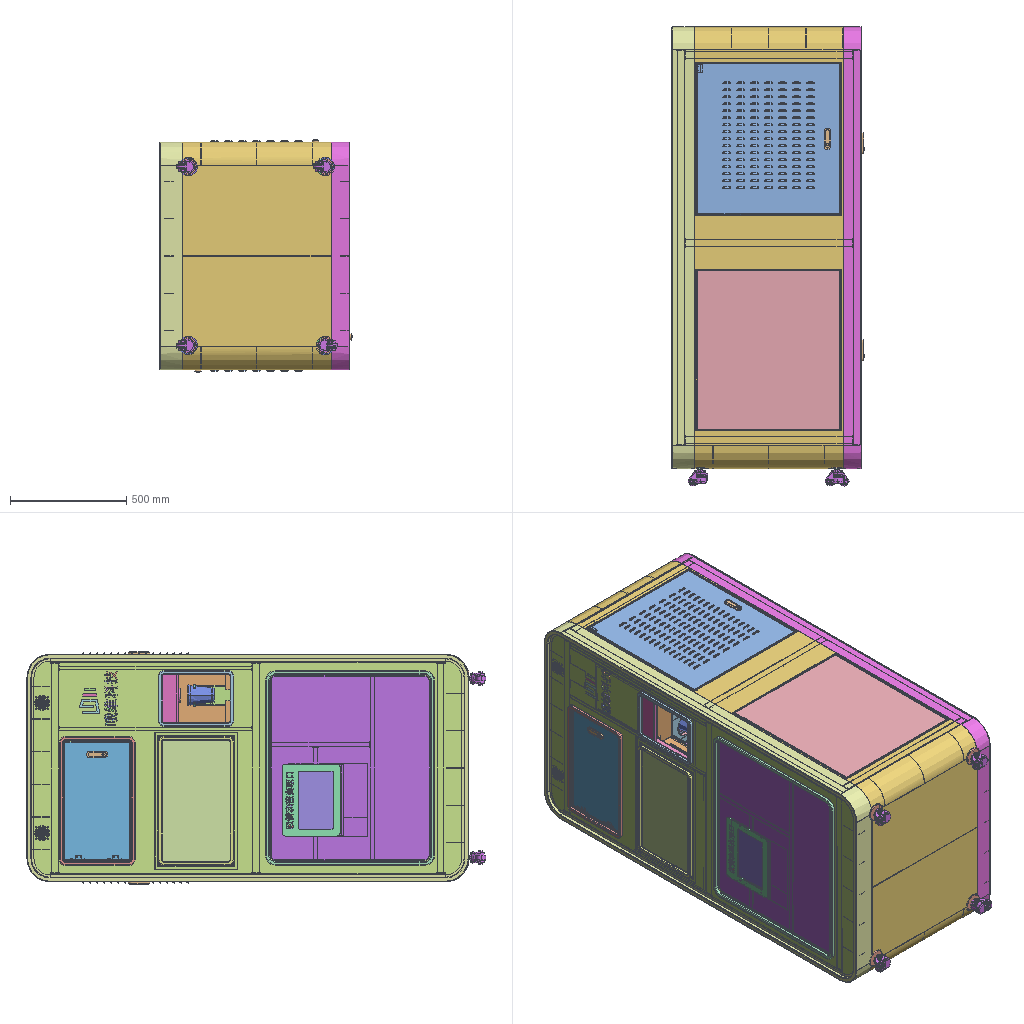Assembly | STEP file | 137 different items | 347 placed | box 826 x 1977 x 1000 mm
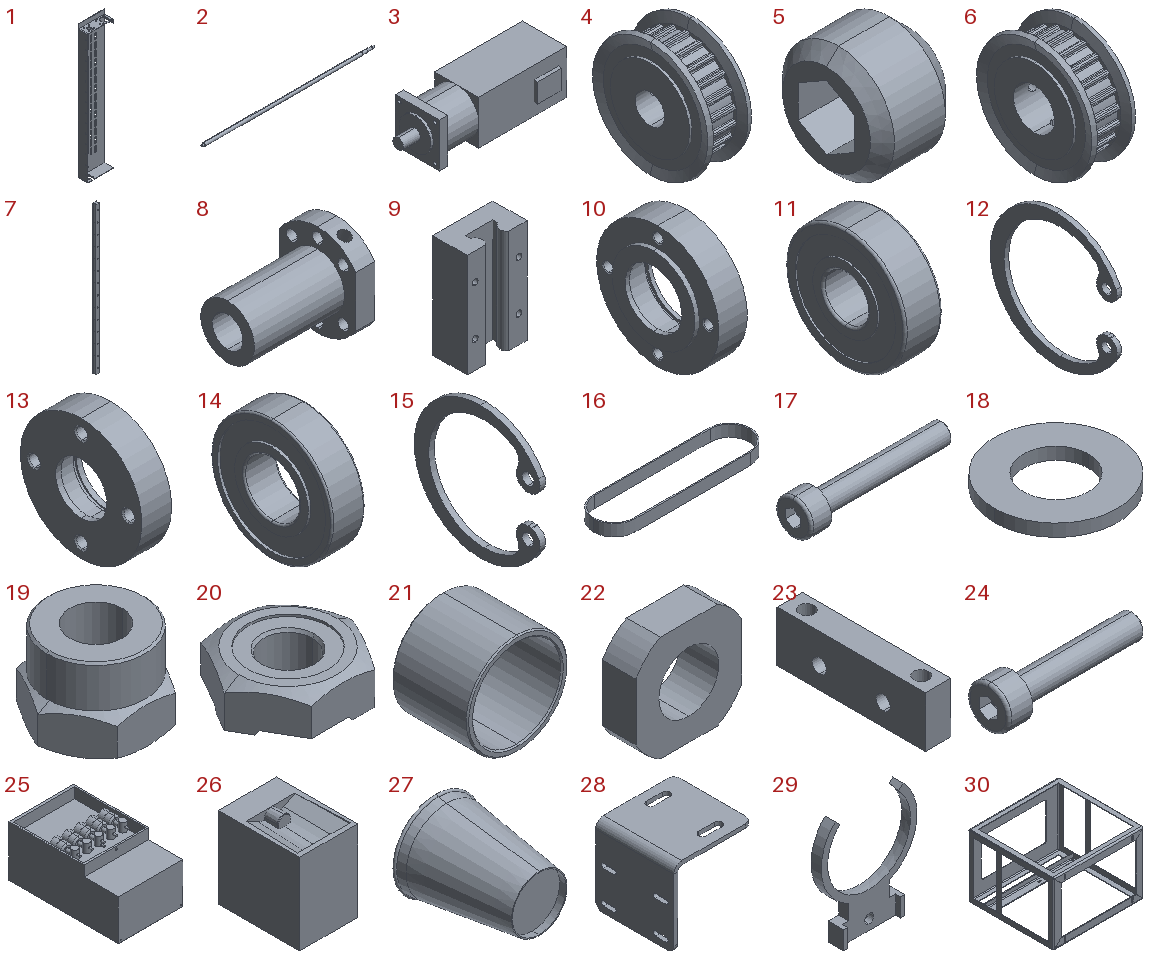Parts list (item | name | quantity | parent item | size | volume):
1 | Lead screw mechanism sheet metal V1.201001 | x1 | in Translation drive module V1.201001 | 175 x 65 x 885 mm | 405761 mm3
2 | Lead screw 16V1.201001 | x1 | in Translation drive module V1.201001 | 882 x 16 x 16 mm | 170889 mm3
3 | PX57N005S0 planetary reducer+motor V1.201001 | x1 | in Translation drive module V1.201001 | 193 x 63 x 58 mm | 546492 mm3
4 | Synchronous wheel TTPA22-AT5100-A-P10_b V1.201001 | x1 | in Synchronous wheel TTPA22-AT5100-A-P10 V1.201001 | 15 x 40 x 40 mm | 11899 mm3
5 | Synchronous wheel SET-SCREW4-3V1.201001 | x2 | in Synchronous wheel TTPA22-AT5100-A-P10 V1.201001 | 3 x 4 x 4 mm | 27.73 mm3
6 | Synchronous wheel shaft 14V1.201001 | x1 | in Translation drive module V1.201001 | 15 x 40 x 40 mm | 10801 mm3
7 | Linear guide rail HG20 V1.201001 | x1 | in Translation drive module V1.201001 | 20 x 18 x 840 mm | 247602 mm3
8 | Lead screw nut SFU01610-3V1.201001 | x1 | in Translation drive module V1.201001 | 57 x 40 x 48 mm | 32254 mm3
9 | Linear slider HGH20CA V1.201001 | x1 | in Translation drive module V1.201001 | 44 x 25 x 76 mm | 66387 mm3
10 | Bearing seat BARR6201DD_b V1.201001 | x1 | in Round flange bearing seat BARR6201 V1.201001 | 15 x 56 x 56 mm | 21210 mm3
11 | Bearing seat bearing_6201 V1.201001 | x1 | in Round flange bearing seat BARR6201 V1.201001 | 10 x 32 x 32 mm | 6608 mm3
12 | Bearing seat RRING-C-INT-32V1.201001 | x1 | in Round flange bearing seat BARR6201 V1.201001 | 1.2 x 32.2 x 33.7 mm | 309.422 mm3
13 | Bearing seat BGRAB6900DD_h V1.201001 | x1 | in Round flange bearing seat BGRAB6900 V1.201001 | 11 x 45 x 45 mm | 12216 mm3
14 | Bearing seat bearing_6900 V1.201001 | x1 | in Round flange bearing seat BGRAB6900 V1.201001 | 6 x 22 x 22 mm | 1661 mm3
15 | Bearing seat RRING-C-INT-22V1.201001 | x1 | in Round flange bearing seat BGRAB6900 V1.201001 | 1 x 21.856 x 23 mm | 128.626 mm3
16 | Belt V1.201001 | x1 | in Translation drive module V1.201001 | 136 x 36 x 10 mm | 3100 mm3
17 | hexagon socket head cap screws gbV1.201001_GB_FASTENER_SCREWS_HSHCS M4X25-N | x3 | in Translation drive module V1.201001 | 29 x 7 x 7 mm | 449.083 mm3
18 | plain washers-n series-grade a gbV1.201001_GB_FASTENER_WASHER_PWNA 5 | x4 | in Translation drive module V1.201001, Coffee machine | 10 x 10 x 1 mm | 56.478 mm3
19 | prevailing torque type style 1 gbV1.201001_GB_HEXAGON_TYPE9 M5-N | x4 | in Translation drive module V1.201001, Coffee machine | 9.238 x 8 x 6.8 mm | 245.877 mm3
20 | hexagon weld nuts gb01001_GB_FASTENER_NUT_JSCN M5-N | x2 | in Translation drive module V1.201001 | 11.547 x 10 x 4 mm | 240.353 mm3
21 | Lead screw shaft end spacer V1.201001 | x1 | in Translation drive module V1.201001 | 16 x 12 x 16 mm | 561.717 mm3
22 | - | x1 | in Translation drive module V1.201001 | 22 x 8 x 22 mm | 2378 mm3
23 | Belt tensioner seat 1001 | x1 | in Translation drive module V1.201001 | 6 x 35 x 12 mm | 2186 mm3
24 | Hex socket cap screw M4 X 20_GB_FASTENER_SCREWS_HSHCS M4X20-N | x1 | in Translation drive module V1.201001 | 24 x 7 x 7 mm | 386.251 mm3
25 | Beverage coffee machine V1.201001 | x1 | in Coffee machine | 430 x 730 x 364 mm | 89425555 mm3
26 | Ice maker V1.201001 | x2 | in Coffee machine | 250 x 350 x 351.956 mm | 29308107 mm3
27 | Paper cup V1.201001 | x2 | in Coffee machine | 92.598 x 112 x 92.598 mm | 30103 mm3
28 | Drive module fixing part V1.201001 | x2 | in Coffee machine | 60 x 60 x 59 mm | 23708 mm3
29 | Cup gripper V1.201001 | x1 | in Coffee machine | 94 x 15 x 108.734 mm | 27097 mm3
30 | Ice maker bracket V1.201001 | x1 | in Coffee machine | 360 x 340 x 250 mm | 395832 mm3
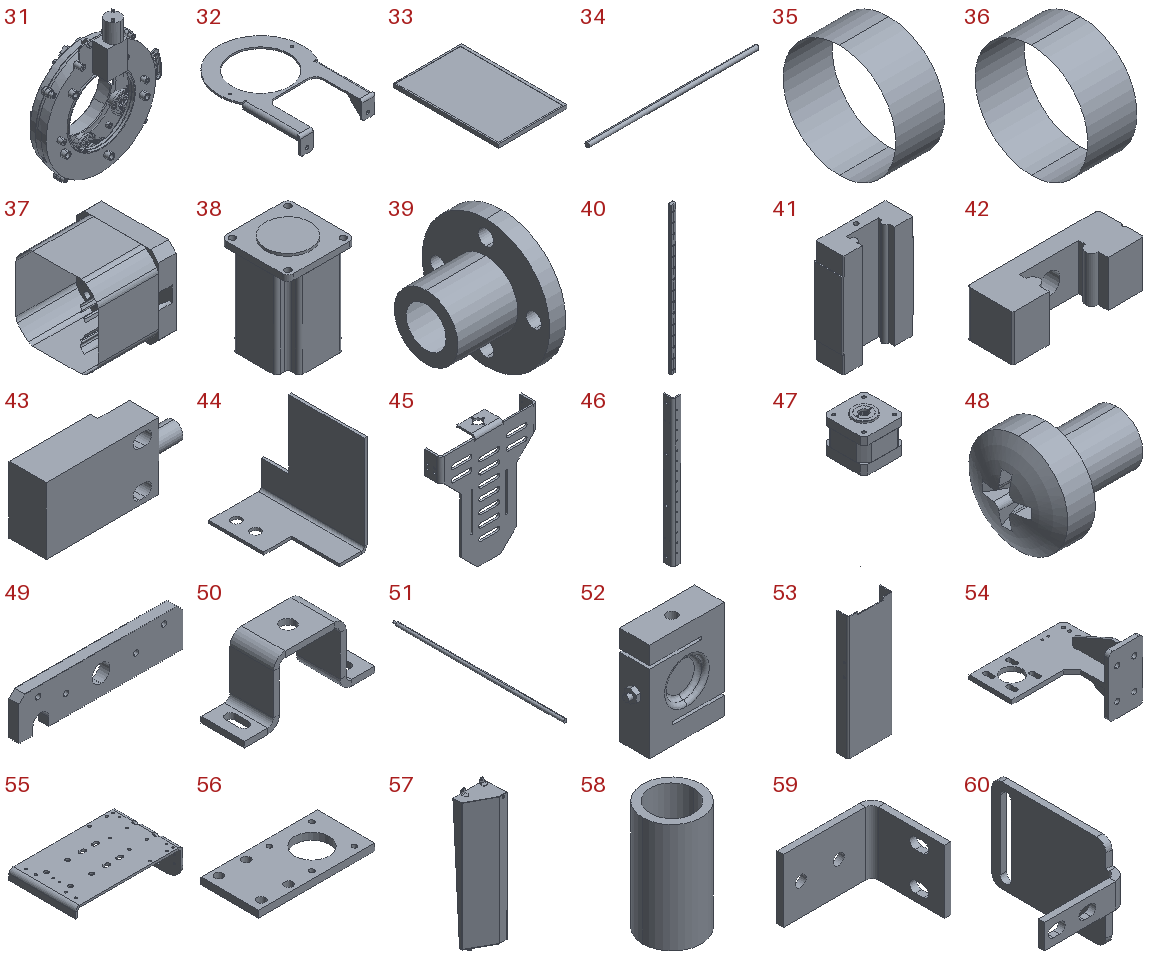31 | 90-bore adjustable cup dropper with cup bucket assembly V1.201001 | x1 | in Coffee machine | - | 341072 mm3
32 | Cup dropper fixing bracket V1.201001 | x1 | in Coffee machine | 160 x 225.6 x 35 mm | 51040 mm3
33 | Operation moving screen V1.201001 | x1 | in Coffee machine | 232 x 356 x 12.5 mm | 957215 mm3
34 | Lift screen drive 42-48-T8-100L_1 V1.201001 | x1 | in Lift screen drive 42-48-T8-100L V1.201001 | - | -
35 | Lift screen drive 42-48-T8-100L_3 V1.201001 | x1 | in Lift screen drive 42-48-T8-100L V1.201001 | - | -
36 | Lift screen drive 42-48-T8-100L_4 V1.201001 | x1 | in Lift screen drive 42-48-T8-100L V1.201001 | - | -
37 | Lift screen drive 42-48-T8-100L_6 V1.201001 | x1 | in Lift screen drive 42-48-T8-100L V1.201001 | - | -
38 | 57 stepper motor 001 | x1 | in Lift screen drive 42-48-T8-100L V1.201001 | 57 x 57 x 80 mm | 221641 mm3
39 | Lead screw nut T10001 | x1 | in Lift screen drive 42-48-T8-100L V1.201001 | - | -
40 | MANIFOLD_SOLID_BREP_106V1.201001 | x2 | in MGN9CV1.201001 | 9 x 6.5 x 300 mm | 14670 mm3
41 | MGN9C slider V1.201001 | x4 | in MGN9CV1.201001, MGN9C for cup gripper 1001, Coffee machine | 20 x 8 x 28.9 mm | 3300 mm3
42 | MGN9 limit block 1001 | x4 | in MGN9CV1.201001 | 20 x 7 x 7 mm | 695.088 mm3
43 | Photoelectric proximity switch V1.201001 | x4 | in Coffee machine | 38.5 x 10.5 x 18.5 mm | 5130 mm3
44 | Proximity switch bracket 3V1.201001 | x1 | in Coffee machine | 20 x 37.5 x 36 mm | 1594 mm3
45 | Lift screen fixing plate V1.201001 | x1 | in Coffee machine | 211 x 40 x 250 mm | 134618 mm3
46 | Guide rail bracket V1.201001 | x2 | in Coffee machine | 18 x 22 x 330 mm | 34095 mm3
47 | 42HSC1409-250NE2V1.201001 | x1 | in Through-type lead screw motor 42HSC1409-250NE2 V1.201001 | 42.3 x 47.3 x 139 mm | 58209 mm3
48 | cross recessed pan head screws gb_GB_CROSS_SCREWS_TYPE1 M3X4-4  H type-NV1.201001 | x4 | in Through-type lead screw motor 42HSC1409-250NE2 V1.201001 | 6.37 x 5.6 x 5.6 mm | 73.791 mm3
49 | Load cell connecting block V1.201001 | x1 | in Coffee lift drive module V1.201001 | 82 x 5 x 20 mm | 7453 mm3
50 | Lead screw connecting block V1.201001 | x1 | in Coffee lift drive module V1.201001 | 45 x 15 x 22 mm | 2255 mm3
51 | Tr8 lead screw V1.201001 | x1 | in Coffee lift drive module V1.201001 | 8 x 388 x 8 mm | 19201 mm3
52 | Load cell JLBS-1V1.201001 | x1 | in Coffee machine | 56 x 20 x 66 mm | 60086 mm3
53 | Upper stop plate V1.201001 | x1 | in Coffee machine | 86 x 23 x 240 mm | 45312 mm3
54 | Lead screw guide rail connecting plate split 1V1.201001 | x1 | in Coffee machine | 110 x 92.5 x 70 mm | 52117 mm3
55 | Lead screw guide rail connecting plate split 2V1.201001 | x1 | in Coffee machine | 161 x 100 x 44.931 mm | 60540 mm3
56 | Lead screw motor drive mounting plate split V1.201001 | x1 | in Coffee machine | 85 x 42 x 5 mm | 14638 mm3
57 | Sink bevel V1.201001 | x1 | in Coffee machine sink bevel V1.201001 | 200 x 147.478 x 872.907 mm | 358159 mm3
58 | Drain pipe weld joint V1.201001 | x1 | in Coffee machine sink bevel V1.201001 | 16 x 16 x 30 mm | 2639 mm3
59 | Cup gripper lift proximity switch bracket 01V1.201001 | x1 | in Coffee machine | 30 x 25 x 20 mm | 1957 mm3
60 | Cup gripper lift proximity switch bracket 02V1.201001 | x1 | in Coffee machine | 27 x 42 x 30 mm | 2421 mm3
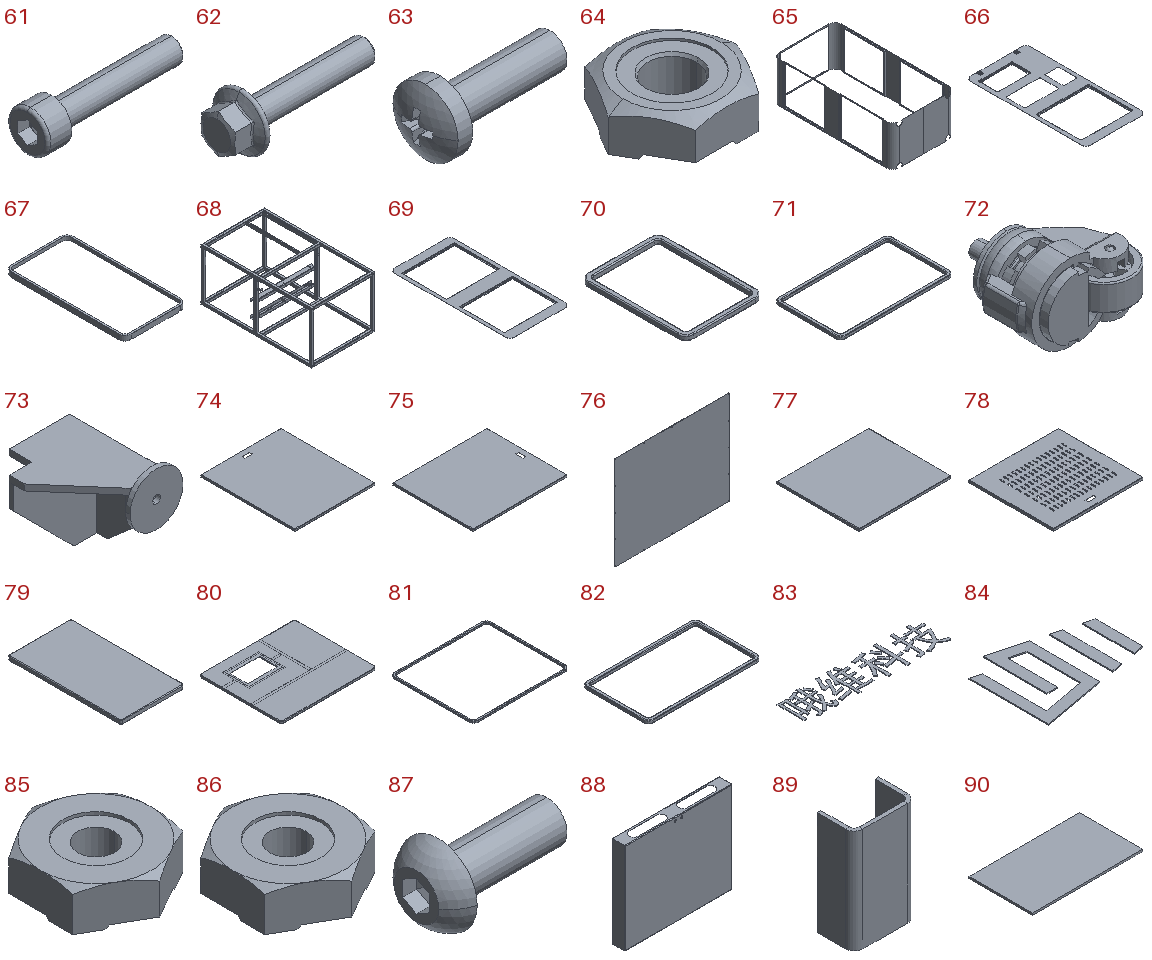61 | hexagon socket head cap screws gbV1.201001_GB_FASTENER_SCREWS_HSHCS M5X25-N | x1 | in Coffee machine | 30 x 8.5 x 8.5 mm | 732.65 mm3
62 | hexagon flange bolts--small series gbV1.201001_GB_FASTENER_BOLT_HFBSS M5X25-N | x1 | in Coffee machine | 30.6 x 11.4 x 11.4 mm | 799.257 mm3
63 | cross recessed pan head screws gbV1.201001_GB_CROSS_SCREWS_TYPE1 M5X16-16  H type-N | x4 | in Coffee machine | 19.658 x 9.5 x 9.5 mm | 509.153 mm3
64 | hexagon weld nuts gbV1.201001_GB_FASTENER_NUT_JSCN M5-N | x2 | in Coffee machine | 11.547 x 10 x 4 mm | 240.353 mm3
65 | Split housing part 0101001 | x1 | in Split arc housing 01001 | 980 x 1900 x 640 mm | 2630768 mm3
66 | Split housing part 0201001 | x1 | in Split arc housing 01001 | 920 x 1840 x 21.5 mm | 1371751 mm3
67 | Split housing part 0301001 | x1 | in Split arc housing 01001 | 980 x 1900 x 80 mm | 894741 mm3
68 | Coffee machine structure frame 01001_default<by machining> | x1 | in Split arc housing 01001 | 977 x 1697 x 797 mm | 7192337 mm3
69 | Split housing part 0401001 | x1 | in Split arc housing 01001 | 920 x 1840 x 21.5 mm | 1137707 mm3
70 | Lift screen decorative outer frame 001001 | x1 | in Split arc housing 01001 | 240 x 325 x 16 mm | 57771 mm3
71 | 23.6 inch transparent screen outer fixing frame 001001 | x1 | in Split arc housing 01001 | 554 x 325 x 16 mm | 92756 mm3
72 | Fuma wheel 60S01001 | x4 | in Split arc housing 01001 | 82.6 x 87.32 x 58 mm | 125258 mm3
73 | Foot support 01001 | x4 | in Split arc housing 01001 | 129 x 131 x 129 mm | 250060 mm3
74 | Rear door panel V1.201001 | x1 | in Split arc housing 01001 | 686 x 805 x 19 mm | 939207 mm3
75 | Rear door panel lower V1.201001 | x1 | in Split arc housing 01001 | 805 x 686 x 19 mm | 939207 mm3
76 | Top cover plate V1.201001 | x1 | in Split arc housing 01001 | 780 x 1.5 x 640 mm | 748466 mm3
77 | Side door panel lower V1.201001 | x2 | in Split arc housing 01001 | 686 x 615 x 19 mm | 731060 mm3
78 | Side door panel upper V1.201001 | x2 | in Split arc housing 01001 | 651 x 615 x 25 mm | 711845 mm3
79 | Front small door panel V1.201001 | x1 | in Split arc housing 01001 | 285 x 511 x 19 mm | 277788 mm3
80 | Front door panel lower V1.201001_default<by machining> | x1 | in Split arc housing 01001 | 796 x 686 x 21.5 mm | 1058682 mm3
81 | Front door outer fixing frame lower 01001 | x1 | in Split arc housing 01001 | 836 x 726 x 16 mm | 745654 mm3
82 | Front small door fixing frame 01001 | x1 | in Split arc housing 01001 | 554 x 325 x 16 mm | 92756 mm3
83 | COMPANY_A 01001 | x1 | in Split arc housing 01001 | 232.982 x 55.205 x 1 mm | 4335 mm3
84 | COMPANY_A LOGO01001 | x1 | in Split arc housing 01001 | 110 x 87.475 x 1 mm | 3655 mm3
85 | Hex weld nut M3_DIN 929-M3-N | x16 | in Split arc housing 01001 | 7.5 x 8.66 x 3 mm | 111.431 mm3
86 | Hex weld nut M3_DIN 929-M3-N | x48 | in Split arc housing 01001 | 7.5 x 8.66 x 3 mm | 111.431 mm3
87 | Hex socket flat round head screw M3 X 8_GB_SOCKET_TYPE7 M3X8-N | x16 | in Split arc housing 01001 | 9.65 x 5.7 x 5.7 mm | 82.74 mm3
88 | Electrical cabinet V1.201001 | x1 | in Split arc housing 01001 | 813 x 100 x 693 mm | 1252271 mm3
89 | Reinforcing rib 1001 | x6 | in Split arc housing 01001 | 25 x 15 x 42 mm | 3127 mm3
90 | 23.6 inch glass 001 | x1 | in Split arc housing 01001 | 550 x 315 x 10 mm | 1732500 mm3
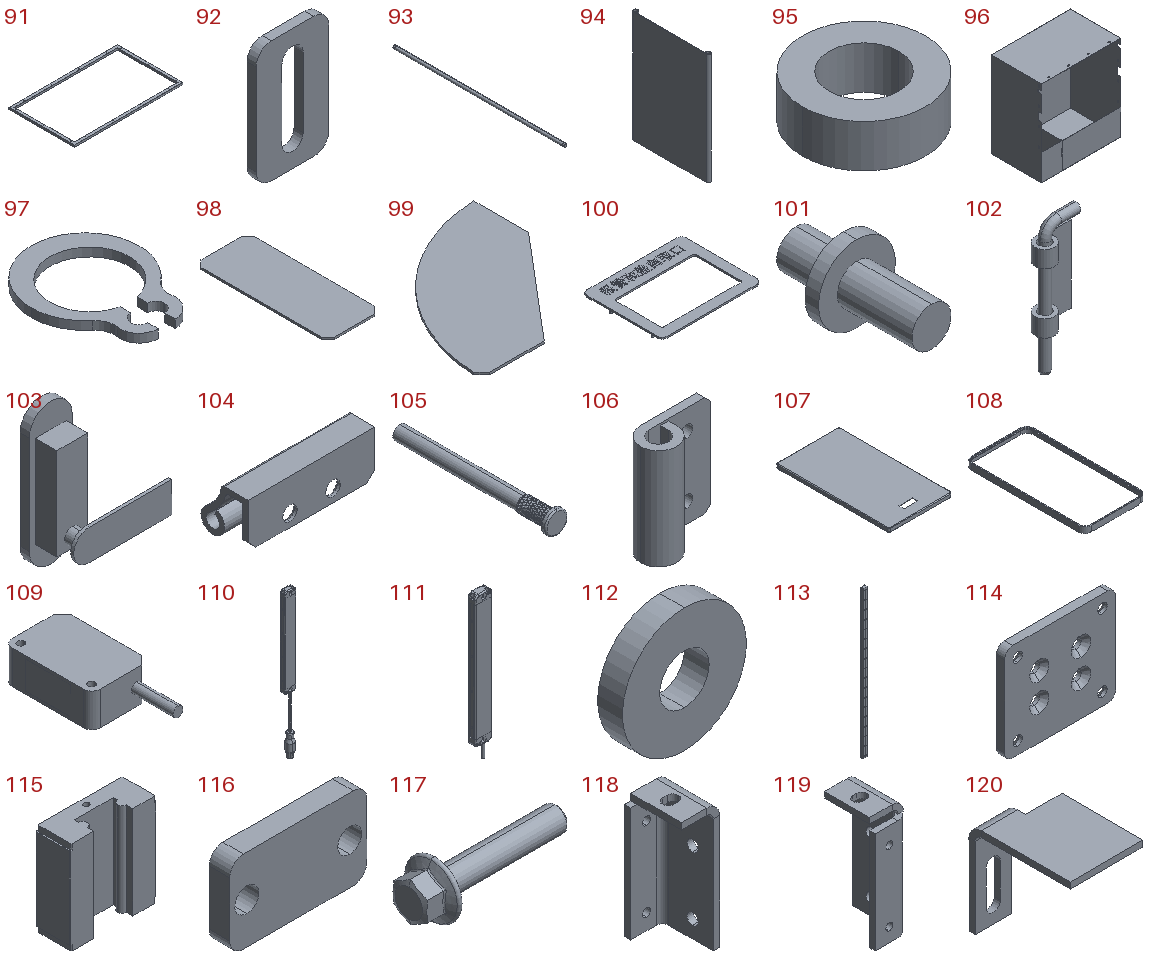91 | Glass mouth reinforcing frame 001 | x1 | in Split arc housing 01001 | 590 x 355 x 11 mm | 93227 mm3
92 | Glass fixing block 001 | x14 | in Split arc housing 01001 | 12 x 1.5 x 20 mm | 277.146 mm3
93 | 6mm pin shaft 001 | x1 | in Split arc housing 01001 | 6 x 320 x 6 mm | 9038 mm3
94 | Coffee machine cover door panel 001 | x1 | in Split arc housing 01001 | 10 x 180 x 260 mm | 84055 mm3
95 | Flip door spacer 001 | x2 | in Split arc housing 01001 | 11.5 x 11.5 x 4 mm | 282.743 mm3
96 | Lid storage box 001 | x1 | in Split arc housing 01001 | 315 x 200 x 340 mm | 428432 mm3
97 | circlips for shaft--type a small gb001_GB_CONNECTING_PIECE_RING_RRA 6 | x2 | in Split arc housing 01001 | 7.6 x 9.565 x 0.6 mm | 14.427 mm3
98 | Box reinforcing rib plate 001 | x22 | in Split arc housing 01001 | 40 x 100 x 1.5 mm | 5925 mm3
99 | Box reinforcing rib plate 2001 | x16 | in Split arc housing 01001 | 94.931 x 99.938 x 1.5 mm | 8426 mm3
100 | Straw and lid self-pickup opening 001 | x1 | in Split arc housing 01001 | 310 x 250 x 20.1 mm | 200534 mm3
101 | Hinge lower door shaft 001 | x4 | in Split arc housing 01001 | 7.8 x 13.8 x 7.8 mm | 219.742 mm3
102 | Latch hinge 001 | x4 | in Split arc housing 01001 | 17.5 x 10 x 55 mm | 2208 mm3
103 | Door lock KL-MS77-1001 | x5 | in Split arc housing 01001 | 68 x 35 x 92 mm | 37880 mm3
104 | - | x2 | in Hinge CL237001 | 48.5 x 18 x 18 mm | 3837 mm3
105 | - | x2 | in Hinge CL237001 | 8 x 57 x 8 mm | 1212 mm3
106 | - | x2 | in Hinge CL237001 | 20 x 9 x 25 mm | 1667 mm3
107 | Front small door panel mating hinge leaf 001 | x1 | in Split arc housing 01001 | 285 x 511 x 19 mm | 270507 mm3
108 | Housing front face solid 001 | x1 | in Split arc housing 01001 | 980 x 1900 x 96 mm | 1146713 mm3
109 | BGS photoelectric switch PG6 V1.201001 | x2 | in Coffee machine | 21 x 46.5 x 12 mm | 7794 mm3
110 | Safety light curtain 4PLN-0440-P V1.201001 | x1 | in Coffee machine | 22.25 x 14.5 x 284 mm | 22094 mm3
111 | Safety light curtain 4PLN-0440V1.201001 | x1 | in Coffee machine | 22 x 10 x 192 mm | 17011 mm3
112 | Guide rail bracket shim 1001 | x7 | in Coffee machine | 10 x 2 x 10 mm | 131.947 mm3
113 | MGN9 guide rail 1001 | x2 | in MGN9C for cup gripper 1001, Coffee machine | 9 x 6.5 x 350 mm | 17052 mm3
114 | MGN9C slider mounting base plate 1001 | x2 | in Coffee machine | 40 x 3 x 35 mm | 3776 mm3
115 | MGN9S slider 1001 | x2 | in Coffee machine | 20 x 8 x 21.5 mm | 2522 mm3
116 | MGN9C short slider pad plate 1001 | x2 | in Coffee machine | 20 x 3 x 12 mm | 651.972 mm3
117 | Hex flange bolt small series M5 X 25_GB_FASTENER_BOLT_HFBSS M5X25-N | x2 | in Coffee machine | 30.6 x 11.4 x 11.4 mm | 799.257 mm3
118 | MGN9 guide rail mounting angle 1001 | x1 | in Coffee machine | 12 x 18 x 40 mm | 2242 mm3
119 | MGN9 guide rail mounting angle mirror part 1001 | x1 | in Coffee machine | 12 x 18 x 40 mm | 2242 mm3
120 | Cup gripper drive lower limit bracket 1001 | x1 | in Coffee machine | 18 x 25 x 23 mm | 825.656 mm3
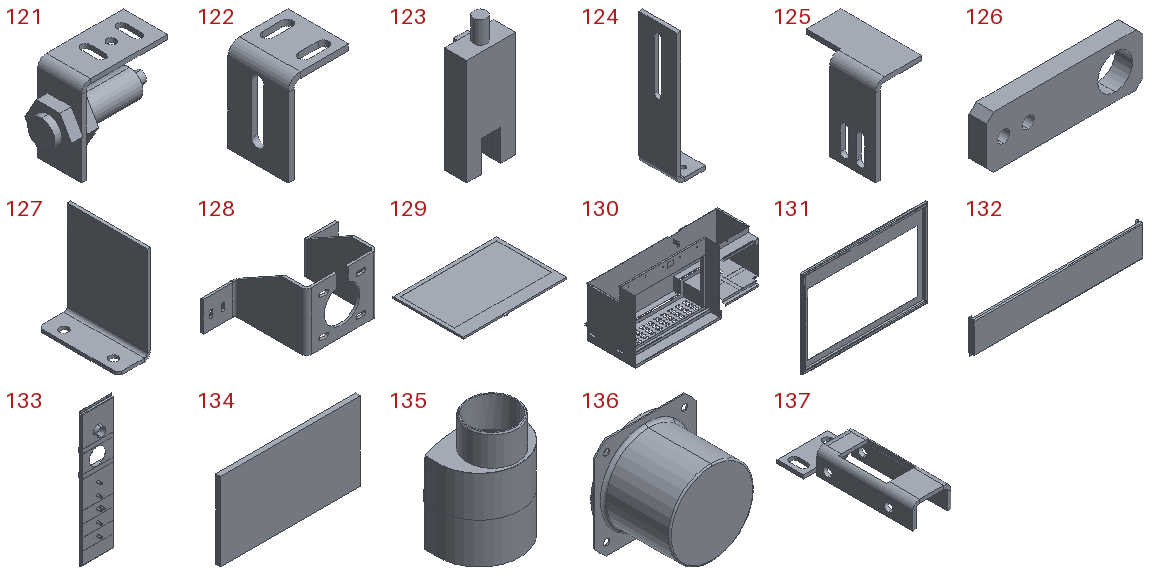121 | M12 laser diffuse reflection sensor 1001 | x1 | in Coffee machine | 46 x 20.785 x 38 mm | 8362 mm3
122 | M12 laser diffuse reflection sensor bracket 1001 | x1 | in Coffee machine | 20 x 20 x 30 mm | 1578 mm3
123 | Slot photoelectric switch FMSM677WR1001 | x7 | in Coffee machine | 13.2 x 13 x 34.5 mm | 2328 mm3
124 | Slot photoelectric switch bracket 1001 | x7 | in Coffee machine | 15 x 20 x 70 mm | 3044 mm3
125 | Slot photoelectric switch sensing plate 1001 | x1 | in Coffee machine | 20 x 35 x 38 mm | 2460 mm3
126 | Extension spring wire fixing bracket 1001 | x1 | in Coffee machine | 45 x 5 x 15 mm | 2846 mm3
127 | Cable fixing bracket 1001 | x1 | in Coffee machine | 20 x 50 x 60 mm | 7568 mm3
128 | Lift screen drive 57 mounting plate 001 | x1 | in Coffee machine | 170 x 93 x 73 mm | 53723 mm3
129 | 23.6 inch screen 01001 | x1 | in Coffee machine | 564 x 390 x 10 mm | 1834790 mm3
130 | Transparent screen built-in cover plate 001 | x1 | in Coffee machine | 926 x 355 x 435 mm | 1573889 mm3
131 | 23.6 inch transparent screen frame 001 | x1 | in Coffee machine | 596 x 13.5 x 414 mm | 232160 mm3
132 | Sealing plate cover 01001 | x1 | in Coffee machine | 599 x 20 x 120.5 mm | 137683 mm3
133 | Sealing plate cover 02001 | x1 | in Coffee machine | 220 x 80 x 922 mm | 432761 mm3
134 | Light guide plate 001 | x1 | in Coffee machine | 590 x 20 x 330 mm | 3894000 mm3
135 | Ice maker outlet adapter 001 | x1 | in Coffee machine | 80.19 x 62.19 x 110 mm | 80643 mm3
136 | Speaker 001 | x2 | in Coffee machine | 67 x 47.8 x 67 mm | 121623 mm3
137 | Cup proximity switch bracket 001 | x1 | in Coffee machine | 21 x 54 x 11.5 mm | 1886 mm3
Placements (level | parent | child | x y z in mm | rotation matrix by rows), first 206 of 361 lines:
1 | Coffee machine | Translation drive module V1.201 | -105.767 -90.835 -457.251 | 1 0 0 0 1 0 0 0 1
2 | Translation drive module V1.201 | Lead screw mechanism sheet metal V1.201 | -6.733 55.835 -1.04 | 1 0 0 0 1 0 0 0 1
2 | Translation drive module V1.201 | Lead screw 16V1.201 | 32.767 85.835 -430.04 | 0 0.5413 -0.8408 0 0.8408 0.5413 1 0 0
2 | Translation drive module V1.201 | PX57N005S0 planetary reducer+motor V1.201 | 132.767 85.835 374.96 | 0 0 1 0 1 0 -1 0 0
2 | Translation drive module V1.201 | Synchronous wheel TTPA22-AT5100-A-P10 V1.201 | 32.767 85.835 453.46 | 0 0.9678 0.2518 0 0.2518 -0.9678 -1 0 0
3 | Synchronous wheel TTPA22-AT5100-A-P10 V1.201 | Synchronous wheel TTPA22-AT5100-A-P10_b V1.201 | -0.0 -0.0 -0.0 | 1 0 0 0 1 0 0 0 1
3 | Synchronous wheel TTPA22-AT5100-A-P10 V1.201 | Synchronous wheel SET-SCREW4-3V1.201 | 8.25 5.0 -0.0 | 0 0 -1 -1 0 0 0 1 -0
3 | Synchronous wheel TTPA22-AT5100-A-P10 V1.201 | Synchronous wheel SET-SCREW4-3V1.201 | 8.25 -0.7116 -4.949 | 0 0 -1 0.1423 0.9898 0 0.9898 -0.1423 0
2 | Translation drive module V1.201 | Synchronous wheel shaft 14V1.201 | 132.767 85.835 453.46 | 0 0.4797 0.8775 0 0.8775 -0.4797 -1 0 0
2 | Translation drive module V1.201 | Linear guide rail HG20 V1.201 | -6.733 68.835 0.9603 | 0 -1 0 1 0 0 0 0 1
2 | Translation drive module V1.201 | Lead screw nut SFU01610-3V1.201 | 32.767 85.835 317.251 | 0 1 0 0 0 1 1 0 0
2 | Translation drive module V1.201 | Linear slider HGH20CA V1.201 | -24.233 68.835 319.751 | 0 -1 0 1 0 0 0 0 1
2 | Translation drive module V1.201 | Round flange bearing seat BARR6201 V1.201 | 32.767 85.835 409.96 | 0 -0.7071 0.7071 0 -0.7071 -0.7071 1 0 -0
3 | Round flange bearing seat BARR6201 V1.201 | Bearing seat BARR6201DD_b V1.201 | -0.0 -0.0 -0.0 | 1 0 0 0 1 0 0 0 1
3 | Round flange bearing seat BARR6201 V1.201 | Bearing seat bearing_6201 V1.201 | 12.0 0.0 -0.0 | -1 0 0 0 -1 0 0 0 1
3 | Round flange bearing seat BARR6201 V1.201 | Bearing seat RRING-C-INT-32V1.201 | 12.6 0.0 -0.0 | 1 0 0 0 1 0 0 0 1
2 | Translation drive module V1.201 | Round flange bearing seat BGRAB6900 V1.201 | 32.767 85.835 -423.54 | 0 0.7071 -0.7071 0 -0.7071 -0.7071 -1 0 -0
3 | Round flange bearing seat BGRAB6900 V1.201 | Bearing seat BGRAB6900DD_h V1.201 | -0.0 -0.0 -0.0 | 1 0 0 0 1 0 0 0 1
3 | Round flange bearing seat BGRAB6900 V1.201 | Bearing seat bearing_6900 V1.201 | -3.5 0.0 0.0 | 1 0 0 0 1 0 0 0 1
3 | Round flange bearing seat BGRAB6900 V1.201 | Bearing seat RRING-C-INT-22V1.201 | 3.0 -0.0 -0.0 | 1 0 0 0 1 0 0 0 1
2 | Translation drive module V1.201 | Belt V1.201 | 82.767 85.835 444.51 | 1 0 0 0 1 0 0 0 1
2 | Translation drive module V1.201 | hexagon socket head cap screws gbV1.201_GB_FASTENER_SCREWS_HSHCS M4X25-N | -23.033 68.835 388.96 | 1 0 0 0 1 0 0 0 1
2 | Translation drive module V1.201 | hexagon socket head cap screws gbV1.201_GB_FASTENER_SCREWS_HSHCS M4X25-N | -23.033 68.835 268.96 | 1 0 0 0 1 0 0 0 1
2 | Translation drive module V1.201 | hexagon socket head cap screws gbV1.201_GB_FASTENER_SCREWS_HSHCS M4X25-N | -23.033 68.835 208.96 | 1 0 0 0 1 0 0 0 1
2 | Translation drive module V1.201 | plain washers-n series-grade a gbV1.201_GB_FASTENER_WASHER_PWNA 5 | -3.733 68.835 388.96 | 0 0 1 0 1 0 -1 0 0
2 | Translation drive module V1.201 | plain washers-n series-grade a gbV1.201_GB_FASTENER_WASHER_PWNA 5 | -3.733 68.835 268.96 | 0 0 1 0 1 0 -1 0 0
2 | Translation drive module V1.201 | plain washers-n series-grade a gbV1.201_GB_FASTENER_WASHER_PWNA 5 | -3.733 68.835 208.96 | 0 0 1 0 1 0 -1 0 0
2 | Translation drive module V1.201 | prevailing torque type style 1 gbV1.201_GB_HEXAGON_TYPE9 M5-N | -0.2131 68.835 388.96 | 0 0 1 0 1 0 -1 0 0
2 | Translation drive module V1.201 | prevailing torque type style 1 gbV1.201_GB_HEXAGON_TYPE9 M5-N | -1.213 68.835 268.96 | 0 0 1 0 1 0 -1 0 0
2 | Translation drive module V1.201 | prevailing torque type style 1 gbV1.201_GB_HEXAGON_TYPE9 M5-N | -1.213 68.835 208.96 | 0 0 1 0 1 0 -1 0 0
2 | Translation drive module V1.201 | hexagon weld nuts gb01001_GB_FASTENER_NUT_JSCN M5-N | 53.267 114.835 421.46 | 1 0 0 0 0 -1 0 1 0
2 | Translation drive module V1.201 | hexagon weld nuts gb01001_GB_FASTENER_NUT_JSCN M5-N | 13.267 114.835 421.46 | 1 0 0 0 0 -1 0 1 0
2 | Translation drive module V1.201 | Lead screw shaft end spacer V1.201 | 32.767 85.835 411.96 | 0.9923 0 0.1235 -0.1235 0 0.9923 0 -1 0
2 | Translation drive module V1.201 | subassembly 2 | 32.767 85.835 391.96 | 1 0 0 0 0 -1 0 1 0
2 | Translation drive module V1.201 | Belt tensioner seat 1001 | 96.267 85.835 426.96 | -1 0 0 0 -1 0 0 0 1
2 | Translation drive module V1.201 | Hex socket cap screw M4 X 20_GB_FASTENER_SCREWS_HSHCS M4X20-N | 79.767 78.335 419.96 | 1 0 0 0 0.9835 -0.1811 0 0.1811 0.9835
1 | Coffee machine | Beverage coffee machine V1.201 | -2.5 525.0 -603.5 | 0 0 -1 0 1 0 1 0 0
1 | Coffee machine | Ice maker V1.201 | 43.5 500.0 -206.5 | -1 0 0 0 1 0 0 0 -1
1 | Coffee machine | Paper cup V1.201 | -226.0 321.642 -291.5 | 1 0 0 0 1 0 0 0 1
1 | Coffee machine | Drive module fixing part V1.201 | -72.5 30.0 -898.5 | 0 -1 0 0 0 -1 1 0 -0
1 | Coffee machine | Drive module fixing part V1.201 | -72.5 30.0 -1.5 | 0 1 0 0 0 -1 -1 0 0
1 | Coffee machine | Cup gripper V1.201 | -226.0 285.0 -137.5 | 0 0 -1 0 1 0 1 0 0
1 | Coffee machine | Paper cup V1.201 | -226.0 195.23 -137.5 | 0 0 -1 0 1 0 1 0 -0
1 | Coffee machine | Ice maker bracket V1.201 | 43.5 500.0 -206.5 | 0 0 1 0 1 0 -1 0 0
1 | Coffee machine | 90-bore adjustable cup dropper with cup bucket assembly V1.201 | -223.246 428.642 -293.022 | 0 0 1 0 1 0 -1 0 0
1 | Coffee machine | Cup dropper fixing bracket V1.201 | -223.246 402.0 -293.022 | 0 -1 0 0 0 -1 1 0 0
1 | Coffee machine | Operation moving screen V1.201 | -440.25 528.0 -151.0 | 0 0 -1 0 1 0 1 0 -0
1 | Coffee machine | Lift screen drive 42-48-T8-100L V1.201 | -410.0 768.5 -151.0 | 0 -1 0 1 0 0 0 0 1
2 | Lift screen drive 42-48-T8-100L V1.201 | Lift screen drive 42-48-T8-100L_1 V1.201 | -0.0 -0.0 -0.0 | 1 0 0 0 1 0 0 0 1
2 | Lift screen drive 42-48-T8-100L V1.201 | Lift screen drive 42-48-T8-100L_3 V1.201 | -0.0 -0.0 -0.0 | 1 0 0 0 1 0 0 0 1
2 | Lift screen drive 42-48-T8-100L V1.201 | Lift screen drive 42-48-T8-100L_4 V1.201 | -0.0 -0.0 -0.0 | 1 0 0 0 1 0 0 0 1
2 | Lift screen drive 42-48-T8-100L V1.201 | Lift screen drive 42-48-T8-100L_6 V1.201 | -0.0 -0.0 -0.0 | 1 0 0 0 1 0 0 0 1
2 | Lift screen drive 42-48-T8-100L V1.201 | 57 stepper motor 001 | 5.0 0.0 0.0 | 0 0 -1 0 1 0 1 0 0
2 | Lift screen drive 42-48-T8-100L V1.201 | Lead screw nut T10001 | -61.827 0.0 -0.0 | 1 0 0 0 1 0 0 0 1
1 | Coffee machine | MGN9CV1.201 | -412.5 404.25 -35.5 | -1 0 0 0 0 -1 0 -1 -0
2 | MGN9CV1.201 | MANIFOLD_SOLID_BREP_106V1.201 | -0.0 -0.0 -0.0 | 1 0 0 0 1 0 0 0 1
2 | MGN9CV1.201 | MGN9C slider V1.201 | 0.0 0.0 -228.75 | 1 0 0 0 1 0 0 0 1
2 | MGN9CV1.201 | MGN9 limit block 1001 | 0.0 0.0 29.0 | 1 0 0 0 1 0 0 0 1
2 | MGN9CV1.201 | MGN9 limit block 1001 | -0.0 -0.0 -264.0 | 1 0 0 0 1 0 0 0 1
1 | Coffee machine | Photoelectric proximity switch V1.201 | -398.5 398.5 -23.5 | 0 1 0 1 0 0 0 0 -1
1 | Coffee machine | Proximity switch bracket 3V1.201 | -409.0 644.25 -49.5 | 1 0 0 0 1 0 0 0 1
1 | Coffee machine | Lift screen fixing plate V1.201 | -434.0 543.0 -151.0 | 0 1 0 0 0 1 1 0 -0
1 | Coffee machine | Guide rail bracket V1.201 | -403.5 524.25 -35.5 | -1 0 0 0 0 1 0 1 0
1 | Coffee machine | Coffee lift drive module V1.201 | -160.5 -148.0 -137.5 | 0 -1 0 0 0 1 -1 0 -0
2 | Coffee lift drive module V1.201 | Through-type lead screw motor 42HSC1409-250NE2 V1.201 | 2.416 2.537 -140.916 | 1 0 0 0 1 0 0 0 1
3 | Through-type lead screw motor 42HSC1409-250NE2 V1.201 | 42HSC1409-250NE2V1.201 | -2.416 -2.537 106.415 | 1 0 0 0 1 0 0 0 1
3 | Through-type lead screw motor 42HSC1409-250NE2 V1.201 | cross recessed pan head screws gb_GB_CROSS_SCREWS_TYPE1 M3X4-4  H type-NV1.201 | -17.916 12.963 106.516 | 0 0 -1 0 1 0 1 0 0
3 | Through-type lead screw motor 42HSC1409-250NE2 V1.201 | cross recessed pan head screws gb_GB_CROSS_SCREWS_TYPE1 M3X4-4  H type-NV1.201 | 13.084 12.963 106.516 | 0 0 -1 0 1 0 1 0 0
3 | Through-type lead screw motor 42HSC1409-250NE2 V1.201 | cross recessed pan head screws gb_GB_CROSS_SCREWS_TYPE1 M3X4-4  H type-NV1.201 | 13.084 -18.037 106.516 | 0 0 -1 0 1 0 1 0 0
3 | Through-type lead screw motor 42HSC1409-250NE2 V1.201 | cross recessed pan head screws gb_GB_CROSS_SCREWS_TYPE1 M3X4-4  H type-NV1.201 | -17.916 -18.037 106.516 | 0 0 -1 0 1 0 1 0 0
2 | Coffee lift drive module V1.201 | Load cell connecting block V1.201 | -0.0 0.0 357.0 | 1 0 0 0 0 1 0 -1 0
2 | Coffee lift drive module V1.201 | Lead screw connecting block V1.201 | -0.0 0.0 330.0 | 1 0 0 0 -1 0 0 0 -1
2 | Coffee lift drive module V1.201 | Tr8 lead screw V1.201 | -0.0 -0.0 -50.0 | 0.7167 0 -0.6974 -0.6974 0 -0.7167 0 1 0
1 | Coffee machine | Load cell JLBS-1V1.201 | -160.5 242.0 -137.5 | 0 1 0 0 0 -1 -1 0 -0
1 | Coffee machine | Upper stop plate V1.201 | -172.0 154.0 -137.5 | 0 1 0 0 0 1 1 0 0
1 | Coffee machine | Lead screw guide rail connecting plate split 1V1.201 | -73.0 -5.0 -140.0 | 0 1 0 -1 0 0 0 0 1
1 | Coffee machine | Lead screw guide rail connecting plate split 2V1.201 | -142.5 2.0 -137.5 | 0 0 -1 -1 0 0 0 1 -0
1 | Coffee machine | Lead screw motor drive mounting plate split V1.201 | -143.0 -143.0 -137.5 | -1 0 0 0 0 -1 0 -1 -0
1 | Coffee machine | Photoelectric proximity switch V1.201 | -135.25 -161.5 -87.5 | 1 0 0 0 0 1 0 -1 0
1 | Coffee machine | Coffee machine sink bevel V1.201 | -303.5 68.75 -451.769 | 0 0 1 -0.9986 -0.05234 0 0.05234 -0.9986 0
2 | Coffee machine sink bevel V1.201 | Sink bevel V1.201 | -0.0 -0.0 -0.0 | 0 -1 0 0 0 1 -1 0 0
2 | Coffee machine sink bevel V1.201 | Drain pipe weld joint V1.201 | 160.0 -0.0 -0.0 | 0 0 1 0 -1 0 1 0 -0
1 | Coffee machine | Cup gripper lift proximity switch bracket 01V1.201 | -124.5 -143.0 -105.5 | 0 0 1 1 0 0 0 1 -0
1 | Coffee machine | Photoelectric proximity switch V1.201 | -167.25 -129.5 -86.5 | -1 0 0 0 0 -1 0 -1 0
1 | Coffee machine | Cup gripper lift proximity switch bracket 02V1.201 | -127.5 -129.5 -106.5 | 0 -1 0 0 0 -1 1 0 0
1 | Coffee machine | Guide rail bracket V1.201 | -403.5 524.25 -266.5 | -1 0 0 0 0 -1 0 -1 0
1 | Coffee machine | MGN9CV1.201 | -412.5 404.25 -266.5 | 1 0 0 0 0 -1 0 1 0
2 | MGN9CV1.201 | MANIFOLD_SOLID_BREP_106V1.201 | -0.0 -0.0 -0.0 | 1 0 0 0 1 0 0 0 1
2 | MGN9CV1.201 | MGN9C slider V1.201 | 0.0 0.0 -228.75 | 1 0 0 0 1 0 0 0 1
2 | MGN9CV1.201 | MGN9 limit block 1001 | 0.0 0.0 29.0 | 1 0 0 0 1 0 0 0 1
2 | MGN9CV1.201 | MGN9 limit block 1001 | 0.0 -0.0 -264.0 | 1 0 0 0 1 0 0 0 1
1 | Coffee machine | hexagon socket head cap screws gbV1.201_GB_FASTENER_SCREWS_HSHCS M5X25-N | -128.0 -153.0 -122.0 | 0 -1 0 1 0 0 0 0 1
1 | Coffee machine | plain washers-n series-grade a gbV1.201_GB_FASTENER_WASHER_PWNA 5 | -128.0 -139.0 -122.0 | 1 0 0 0 0 1 0 -1 0
1 | Coffee machine | prevailing torque type style 1 gbV1.201_GB_HEXAGON_TYPE9 M5-N | -128.0 -135.48 -122.0 | 1 0 0 0 0 1 0 -1 0
1 | Coffee machine | hexagon flange bolts--small series gbV1.201_GB_FASTENER_BOLT_HFBSS M5X25-N | 52.25 18.5 -22.691 | 0 0 1 0 1 0 -1 0 0
1 | Coffee machine | cross recessed pan head screws gbV1.201_GB_CROSS_SCREWS_TYPE1 M5X16-16  H type-N | -89.263 11.264 -24.591 | 0 0 1 0 1 0 -1 0 0
1 | Coffee machine | cross recessed pan head screws gbV1.201_GB_CROSS_SCREWS_TYPE1 M5X16-16  H type-N | -89.263 -21.264 -24.591 | 0 0 1 0 1 0 -1 0 0
1 | Coffee machine | cross recessed pan head screws gbV1.201_GB_CROSS_SCREWS_TYPE1 M5X16-16  H type-N | -56.736 -21.264 -24.591 | 0 0 1 0 1 0 -1 0 0
1 | Coffee machine | cross recessed pan head screws gbV1.201_GB_CROSS_SCREWS_TYPE1 M5X16-16  H type-N | -56.736 11.264 -24.591 | 0 0 1 0 1 0 -1 0 0
1 | Coffee machine | hexagon weld nuts gbV1.201_GB_FASTENER_NUT_JSCN M5-N | -97.0 125.0 -881.0 | 0 0 -1 0 1 0 1 0 -0
1 | Coffee machine | hexagon weld nuts gbV1.201_GB_FASTENER_NUT_JSCN M5-N | -97.0 125.0 -10.0 | 0 0 -1 -0.02751 0.9996 0 0.9996 0.02751 -0
1 | Coffee machine | Split arc housing 01001 | -50.0 1000.0 -450.0 | 0 0 -1 0 1 0 1 0 -0
2 | Split arc housing 01001 | Split housing part 0101001 | -0.0 -0.0 -0.0 | 1 0 0 0 1 0 0 0 1
2 | Split arc housing 01001 | Split housing part 0201001 | -0.0 -950.0 400.0 | 1 0 0 0 1 0 0 0 1
2 | Split arc housing 01001 | Split housing part 0301001 | -0.0 -950.0 -320.0 | -1 0 0 0 1 0 0 0 -1
2 | Split arc housing 01001 | Coffee machine structure frame 01001_default<by machining> | 0.0 -1798.5 378.5 | 1 0 0 0 1 0 0 0 1
2 | Split arc housing 01001 | Split housing part 0401001 | 0.0 -950.0 -400.0 | -1 0 0 0 1 0 0 0 -1
2 | Split arc housing 01001 | Lift screen decorative outer frame 001001 | 299.0 -727.5 400.0 | 1 0 0 0 1 0 0 0 1
2 | Split arc housing 01001 | 23.6 inch transparent screen outer fixing frame 001001 | -141.0 -727.5 400.0 | 1 0 0 0 1 0 0 0 1
2 | Split arc housing 01001 | Fuma wheel 60S01001 | -384.5 -1904.5 -294.5 | -0.03394 0 0.9994 0 1 0 -0.9994 0 -0.03394
2 | Split arc housing 01001 | Foot support 01001 | -478.5 -1798.5 -274.5 | 1 0 0 0 1 0 0 0 1
2 | Split arc housing 01001 | Foot support 01001 | 364.5 -1798.5 -388.5 | 0 0 -1 0 1 0 1 0 -0
2 | Split arc housing 01001 | Fuma wheel 60S01001 | 384.5 -1904.5 -294.5 | 0.02656 0 -0.9996 0 1 0 0.9996 0 0.02656
2 | Split arc housing 01001 | Foot support 01001 | 478.5 -1798.5 274.5 | -1 0 0 0 1 0 0 0 -1
2 | Split arc housing 01001 | Foot support 01001 | -364.5 -1798.5 388.5 | 0 0 1 0 1 0 -1 0 -0
2 | Split arc housing 01001 | Fuma wheel 60S01001 | 384.5 -1904.5 294.5 | 0.01835 0 -0.9998 0 1 0 0.9998 0 0.01835
2 | Split arc housing 01001 | Fuma wheel 60S01001 | -384.5 -1904.5 294.5 | -0.02357 0 -0.9997 0 1 0 0.9997 0 -0.02357
2 | Split arc housing 01001 | Rear door panel V1.201 | -0.0 -500.0 -400.0 | 0 -1 0 -1 0 0 0 0 -1
2 | Split arc housing 01001 | Rear door panel lower V1.201 | -0.0 -1390.0 -400.0 | -1 0 0 0 1 0 0 0 -1
2 | Split arc housing 01001 | Top cover plate V1.201 | -0.0 -0.0 -0.0 | 1 0 0 0 1 0 0 0 1
2 | Split arc housing 01001 | Side door panel lower V1.201 | -490.0 -1390.0 -0.0 | 0 0 -1 -1 0 0 0 1 0
2 | Split arc housing 01001 | Side door panel lower V1.201 | 490.0 -1390.0 -0.0 | 0 0 1 -1 0 0 0 -1 -0
2 | Split arc housing 01001 | Side door panel upper V1.201 | -490.0 -482.5 -0.0 | 0 0 -1 1 0 0 0 -1 0
2 | Split arc housing 01001 | Side door panel upper V1.201 | 490.0 -482.5 0.0 | 0 0 1 1 0 0 0 1 0
2 | Split arc housing 01001 | Front small door panel V1.201 | -142.0 -302.5 400.0 | 0 1 0 -1 0 0 0 0 1
2 | Split arc housing 01001 | Front door panel lower V1.201_default<by machining> | -0.0 -1390.0 400.0 | 1 0 0 0 1 0 0 0 1
2 | Split arc housing 01001 | Front door outer fixing frame lower 01001 | -0.0 -1390.0 400.0 | 1 0 0 0 1 0 0 0 1
2 | Split arc housing 01001 | Front small door fixing frame 01001 | -142.0 -302.5 416.0 | -1 0 0 0 1 0 0 0 -1
2 | Split arc housing 01001 | COMPANY_A 01001 | 299.0 -382.5 400.0 | 1 0 0 0 1 0 0 0 1
2 | Split arc housing 01001 | COMPANY_A LOGO01001 | 299.0 -272.5 400.0 | 1 0 0 0 1 0 0 0 1
2 | Split arc housing 01001 | Hex weld nut M3_DIN 929-M3-N | -385.0 -3.95 -315.0 | 1 0 0 0 0 -1 0 1 0
2 | Split arc housing 01001 | Hex weld nut M3_DIN 929-M3-N | -385.0 -3.95 -157.5 | 1 0 0 0 0 -1 0 1 0
2 | Split arc housing 01001 | Hex weld nut M3_DIN 929-M3-N | -385.0 -3.95 -0.0 | 1 0 0 0 0 -1 0 1 0
2 | Split arc housing 01001 | Hex weld nut M3_DIN 929-M3-N | -385.0 -3.95 157.5 | 1 0 0 0 0 -1 0 1 0
2 | Split arc housing 01001 | Hex weld nut M3_DIN 929-M3-N | -385.0 -3.95 315.0 | 1 0 0 0 0 -1 0 1 0
2 | Split arc housing 01001 | Hex weld nut M3_DIN 929-M3-N | -192.5 -3.95 -315.0 | 1 0 0 0 0 -1 0 1 0
2 | Split arc housing 01001 | Hex weld nut M3_DIN 929-M3-N | 0.0 -3.95 -315.0 | 1 0 0 0 0 -1 0 1 0
2 | Split arc housing 01001 | Hex weld nut M3_DIN 929-M3-N | 192.5 -3.95 -315.0 | 1 0 0 0 0 -1 0 1 0
2 | Split arc housing 01001 | Hex weld nut M3_DIN 929-M3-N | 385.0 -3.95 -315.0 | 1 0 0 0 0 -1 0 1 0
2 | Split arc housing 01001 | Hex weld nut M3_DIN 929-M3-N | -474.95 -1053.5 270.0 | 0 0 -1 0 1 0 1 0 -0
2 | Split arc housing 01001 | Hex weld nut M3_DIN 929-M3-N | -474.95 -1090.0 301.0 | 0 0 -1 0 1 0 1 0 -0
2 | Split arc housing 01001 | Hex weld nut M3_DIN 929-M3-N | -474.95 -1290.0 301.0 | 0 0 -1 0 1 0 1 0 -0
2 | Split arc housing 01001 | Hex weld nut M3_DIN 929-M3-N | -474.95 -1490.0 301.0 | 0 0 -1 0 1 0 1 0 -0
2 | Split arc housing 01001 | Hex weld nut M3_DIN 929-M3-N | -474.95 -1690.0 301.0 | 0 0 -1 0 1 0 1 0 -0
2 | Split arc housing 01001 | Hex weld nut M3_DIN 929-M3-N | -474.95 -1726.5 270.0 | 0 0 -1 0 1 0 1 0 -0
2 | Split arc housing 01001 | Hex weld nut M3_DIN 929-M3-N | -474.95 -1726.5 100.0 | 0 0 -1 0 1 0 1 0 -0
2 | Split arc housing 01001 | Hex weld nut M3_DIN 929-M3-N | -474.95 -1726.5 -100.0 | 0 0 -1 0 1 0 1 0 -0
2 | Split arc housing 01001 | Hex weld nut M3_DIN 929-M3-N | -474.95 -1726.5 -270.0 | 0 0 -1 0 1 0 1 0 -0
2 | Split arc housing 01001 | Hex weld nut M3_DIN 929-M3-N | -474.95 -1690.0 -301.0 | 0 0 -1 0 1 0 1 0 -0
2 | Split arc housing 01001 | Hex weld nut M3_DIN 929-M3-N | -474.95 -1490.0 -301.0 | 0 0 -1 0 1 0 1 0 -0
2 | Split arc housing 01001 | Hex weld nut M3_DIN 929-M3-N | -474.95 -1290.0 -301.0 | 0 0 -1 0 1 0 1 0 -0
2 | Split arc housing 01001 | Hex weld nut M3_DIN 929-M3-N | -474.95 -1090.0 -301.0 | 0 0 -1 0 1 0 1 0 -0
2 | Split arc housing 01001 | Hex weld nut M3_DIN 929-M3-N | -474.95 -1053.5 -270.0 | 0 0 -1 0 1 0 1 0 -0
2 | Split arc housing 01001 | Hex weld nut M3_DIN 929-M3-N | -474.95 -1053.5 -100.0 | 0 0 -1 0 1 0 1 0 -0
2 | Split arc housing 01001 | Hex weld nut M3_DIN 929-M3-N | -474.95 -1053.5 100.0 | 0 0 -1 0 1 0 1 0 -0
2 | Split arc housing 01001 | Hex weld nut M3_DIN 929-M3-N | 474.95 -1053.5 270.0 | 0 0 1 0 1 0 -1 0 -0
2 | Split arc housing 01001 | Hex weld nut M3_DIN 929-M3-N | 474.95 -1053.5 100.0 | 0 0 1 0 1 0 -1 0 -0
2 | Split arc housing 01001 | Hex weld nut M3_DIN 929-M3-N | 474.95 -1053.5 -100.0 | 0 0 1 0 1 0 -1 0 -0
2 | Split arc housing 01001 | Hex weld nut M3_DIN 929-M3-N | 474.95 -1053.5 -270.0 | 0 0 1 0 1 0 -1 0 -0
2 | Split arc housing 01001 | Hex weld nut M3_DIN 929-M3-N | 474.95 -1090.0 -301.0 | 0 0 1 0 1 0 -1 0 -0
2 | Split arc housing 01001 | Hex weld nut M3_DIN 929-M3-N | 474.95 -1290.0 -301.0 | 0 0 1 0 1 0 -1 0 -0
2 | Split arc housing 01001 | Hex weld nut M3_DIN 929-M3-N | 474.95 -1490.0 -301.0 | 0 0 1 0 1 0 -1 0 -0
2 | Split arc housing 01001 | Hex weld nut M3_DIN 929-M3-N | 474.95 -1690.0 -301.0 | 0 0 1 0 1 0 -1 0 -0
2 | Split arc housing 01001 | Hex weld nut M3_DIN 929-M3-N | 474.95 -1726.5 -270.0 | 0 0 1 0 1 0 -1 0 -0
2 | Split arc housing 01001 | Hex weld nut M3_DIN 929-M3-N | 474.95 -1726.5 -100.0 | 0 0 1 0 1 0 -1 0 -0
2 | Split arc housing 01001 | Hex weld nut M3_DIN 929-M3-N | 474.95 -1726.5 100.0 | 0 0 1 0 1 0 -1 0 -0
2 | Split arc housing 01001 | Hex weld nut M3_DIN 929-M3-N | 474.95 -1726.5 270.0 | 0 0 1 0 1 0 -1 0 -0
2 | Split arc housing 01001 | Hex weld nut M3_DIN 929-M3-N | 474.95 -1690.0 301.0 | 0 0 1 0 1 0 -1 0 -0
2 | Split arc housing 01001 | Hex weld nut M3_DIN 929-M3-N | 474.95 -1490.0 301.0 | 0 0 1 0 1 0 -1 0 -0
2 | Split arc housing 01001 | Hex weld nut M3_DIN 929-M3-N | 474.95 -1290.0 301.0 | 0 0 1 0 1 0 -1 0 -0
2 | Split arc housing 01001 | Hex weld nut M3_DIN 929-M3-N | 474.95 -1090.0 301.0 | 0 0 1 0 1 0 -1 0 -0
2 | Split arc housing 01001 | Hex weld nut M3_DIN 929-M3-N | -300.0 -1053.5 384.95 | 1 0 0 0 1 0 0 0 1
2 | Split arc housing 01001 | Hex weld nut M3_DIN 929-M3-N | -100.0 -1053.5 384.95 | 1 0 0 0 1 0 0 0 1
2 | Split arc housing 01001 | Hex weld nut M3_DIN 929-M3-N | 100.0 -1053.5 384.95 | 1 0 0 0 1 0 0 0 1
2 | Split arc housing 01001 | Hex weld nut M3_DIN 929-M3-N | 300.0 -1053.5 384.95 | 1 0 0 0 1 0 0 0 1
2 | Split arc housing 01001 | Hex weld nut M3_DIN 929-M3-N | 391.5 -1090.0 384.95 | 1 0 0 0 1 0 0 0 1
2 | Split arc housing 01001 | Hex weld nut M3_DIN 929-M3-N | 391.5 -1290.0 384.95 | 1 0 0 0 1 0 0 0 1
2 | Split arc housing 01001 | Hex weld nut M3_DIN 929-M3-N | 391.5 -1490.0 384.95 | 1 0 0 0 1 0 0 0 1
2 | Split arc housing 01001 | Hex weld nut M3_DIN 929-M3-N | 391.5 -1690.0 384.95 | 1 0 0 0 1 0 0 0 1
2 | Split arc housing 01001 | Hex weld nut M3_DIN 929-M3-N | 300.0 -1726.5 384.95 | 1 0 0 0 1 0 0 0 1
2 | Split arc housing 01001 | Hex weld nut M3_DIN 929-M3-N | 100.0 -1726.5 384.95 | 1 0 0 0 1 0 0 0 1
2 | Split arc housing 01001 | Hex weld nut M3_DIN 929-M3-N | -100.0 -1726.5 384.95 | 1 0 0 0 1 0 0 0 1
2 | Split arc housing 01001 | Hex weld nut M3_DIN 929-M3-N | -300.0 -1726.5 384.95 | 1 0 0 0 1 0 0 0 1
2 | Split arc housing 01001 | Hex weld nut M3_DIN 929-M3-N | -391.5 -1690.0 384.95 | 1 0 0 0 1 0 0 0 1
2 | Split arc housing 01001 | Hex weld nut M3_DIN 929-M3-N | -391.5 -1490.0 384.95 | 1 0 0 0 1 0 0 0 1
2 | Split arc housing 01001 | Hex weld nut M3_DIN 929-M3-N | -391.5 -1290.0 384.95 | 1 0 0 0 1 0 0 0 1
2 | Split arc housing 01001 | Hex weld nut M3_DIN 929-M3-N | -391.5 -1090.0 384.95 | 1 0 0 0 1 0 0 0 1
2 | Split arc housing 01001 | Hex weld nut M3_DIN 929-M3-N | 385.0 -3.95 315.0 | -1 0 0 0 0 -1 0 -1 0
2 | Split arc housing 01001 | Hex weld nut M3_DIN 929-M3-N | 192.5 -3.95 315.0 | -1 0 0 0 0 -1 0 -1 0
2 | Split arc housing 01001 | Hex weld nut M3_DIN 929-M3-N | -0.0 -3.95 315.0 | -1 0 0 0 0 -1 0 -1 0
2 | Split arc housing 01001 | Hex weld nut M3_DIN 929-M3-N | -192.5 -3.95 315.0 | -1 0 0 0 0 -1 0 -1 0
2 | Split arc housing 01001 | Hex weld nut M3_DIN 929-M3-N | 385.0 -3.95 -157.5 | 1 0 0 0 0 -1 0 1 0
2 | Split arc housing 01001 | Hex weld nut M3_DIN 929-M3-N | 385.0 -3.95 0.0 | 1 0 0 0 0 -1 0 1 0
2 | Split arc housing 01001 | Hex weld nut M3_DIN 929-M3-N | 385.0 -3.95 157.5 | 1 0 0 0 0 -1 0 1 0
2 | Split arc housing 01001 | Hex socket flat round head screw M3 X 8_GB_SOCKET_TYPE7 M3X8-N | -385.0 3.15 315.0 | 0 1 0 -1 0 0 0 0 1
2 | Split arc housing 01001 | Hex socket flat round head screw M3 X 8_GB_SOCKET_TYPE7 M3X8-N | -192.5 3.15 315.0 | 0 1 0 -1 0 0 0 0 1
2 | Split arc housing 01001 | Hex socket flat round head screw M3 X 8_GB_SOCKET_TYPE7 M3X8-N | 0.0 3.15 315.0 | 0 1 0 -1 0 0 0 0 1
2 | Split arc housing 01001 | Hex socket flat round head screw M3 X 8_GB_SOCKET_TYPE7 M3X8-N | 192.5 3.15 315.0 | 0 1 0 -1 0 0 0 0 1
2 | Split arc housing 01001 | Hex socket flat round head screw M3 X 8_GB_SOCKET_TYPE7 M3X8-N | 385.0 3.15 315.0 | 0 1 0 -1 0 0 0 0 1
2 | Split arc housing 01001 | Hex socket flat round head screw M3 X 8_GB_SOCKET_TYPE7 M3X8-N | 385.0 3.15 157.5 | 0 1 0 -1 0 0 0 0 1
2 | Split arc housing 01001 | Hex socket flat round head screw M3 X 8_GB_SOCKET_TYPE7 M3X8-N | 385.0 3.15 -0.0 | 0 1 0 -1 0 0 0 0 1
2 | Split arc housing 01001 | Hex socket flat round head screw M3 X 8_GB_SOCKET_TYPE7 M3X8-N | 385.0 3.15 -157.5 | 0 1 0 -1 0 0 0 0 1
2 | Split arc housing 01001 | Hex socket flat round head screw M3 X 8_GB_SOCKET_TYPE7 M3X8-N | 385.0 3.15 -315.0 | 0 1 0 -1 0 0 0 0 1
2 | Split arc housing 01001 | Hex socket flat round head screw M3 X 8_GB_SOCKET_TYPE7 M3X8-N | 192.5 3.15 -315.0 | 0 1 0 -1 0 0 0 0 1
2 | Split arc housing 01001 | Hex socket flat round head screw M3 X 8_GB_SOCKET_TYPE7 M3X8-N | 0.0 3.15 -315.0 | 0 1 0 -1 0 0 0 0 1
2 | Split arc housing 01001 | Hex socket flat round head screw M3 X 8_GB_SOCKET_TYPE7 M3X8-N | -192.5 3.15 -315.0 | 0 1 0 -1 0 0 0 0 1